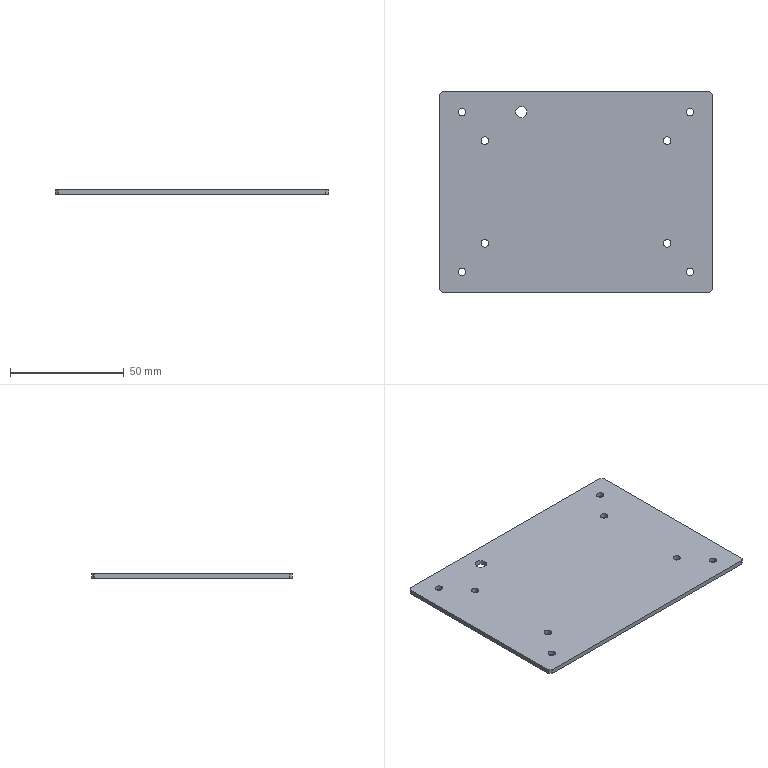Part | SolidWorks | features Extrusion 1, ICE 1 | 1 solid | 28 faces | box 120 x 88 x 2 mm | volume 20938 mm3 | cylinder 22 | plane 6 | commonest cylinder face diameters 3.3 x16 9 x4 5 x2
STEP:
#1=CARTESIAN_POINT('',(-26.5,35.,-1.));
#2=VERTEX_POINT('',#1);
#3=CARTESIAN_POINT('',(-21.5,35.,-1.));
#4=VERTEX_POINT('',#3);
#5=CARTESIAN_POINT('',(-24.,35.,-1.));
#6=DIRECTION('',(0.,0.,1.));
#7=DIRECTION('',(1.,0.,0.));
#8=AXIS2_PLACEMENT_3D('',#5,#6,#7);
#9=CIRCLE('',#8,2.5);
#10=EDGE_CURVE('',#2,#4,#9,.T.);
#11=ORIENTED_EDGE('',*,*,#10,.F.);
#12=CARTESIAN_POINT('',(-26.5,35.,1.));
#13=VERTEX_POINT('',#12);
#14=CARTESIAN_POINT('',(-26.5,35.,-1.));
#15=DIRECTION('',(0.,0.,1.));
#16=VECTOR('',#15,1000.);
#17=LINE('',#14,#16);
#18=EDGE_CURVE('',#2,#13,#17,.T.);
#19=ORIENTED_EDGE('',*,*,#18,.T.);
#20=CARTESIAN_POINT('',(-21.5,35.,1.));
#21=VERTEX_POINT('',#20);
#22=CARTESIAN_POINT('',(-24.,35.,1.));
#23=DIRECTION('',(0.,0.,1.));
#24=DIRECTION('',(1.,0.,0.));
#25=AXIS2_PLACEMENT_3D('',#22,#23,#24);
#26=CIRCLE('',#25,2.5);
#27=EDGE_CURVE('',#13,#21,#26,.T.);
#28=ORIENTED_EDGE('',*,*,#27,.T.);
#29=CARTESIAN_POINT('',(-21.5,35.,-1.));
#30=DIRECTION('',(0.,0.,1.));
#31=VECTOR('',#30,1000.);
#32=LINE('',#29,#31);
#33=EDGE_CURVE('',#4,#21,#32,.T.);
#34=ORIENTED_EDGE('',*,*,#33,.F.);
#35=EDGE_LOOP('',(#11,#19,#28,#34));
#36=FACE_OUTER_BOUND('',#35,.T.);
#37=CARTESIAN_POINT('',(-24.,35.,-1.));
#38=DIRECTION('',(0.,0.,1.));
#39=DIRECTION('',(1.,0.,0.));
#40=AXIS2_PLACEMENT_3D('',#37,#38,#39);
#41=CYLINDRICAL_SURFACE('',#40,2.5);
#42=ADVANCED_FACE('',(#36),#41,.F.);
#43=CARTESIAN_POINT('',(48.35,35.,-1.));
#44=VERTEX_POINT('',#43);
#45=CARTESIAN_POINT('',(51.65,35.,-1.));
#46=VERTEX_POINT('',#45);
#47=CARTESIAN_POINT('',(50.,35.,-1.));
#48=DIRECTION('',(0.,0.,1.));
#49=DIRECTION('',(1.,0.,0.));
#50=AXIS2_PLACEMENT_3D('',#47,#48,#49);
#51=CIRCLE('',#50,1.65);
#52=EDGE_CURVE('',#44,#46,#51,.T.);
#53=ORIENTED_EDGE('',*,*,#52,.F.);
#54=CARTESIAN_POINT('',(48.35,35.,1.));
#55=VERTEX_POINT('',#54);
#56=CARTESIAN_POINT('',(48.35,35.,-1.));
#57=DIRECTION('',(0.,0.,1.));
#58=VECTOR('',#57,1000.);
#59=LINE('',#56,#58);
#60=EDGE_CURVE('',#44,#55,#59,.T.);
#61=ORIENTED_EDGE('',*,*,#60,.T.);
#62=CARTESIAN_POINT('',(51.65,35.,1.));
#63=VERTEX_POINT('',#62);
#64=CARTESIAN_POINT('',(50.,35.,1.));
#65=DIRECTION('',(0.,0.,1.));
#66=DIRECTION('',(1.,0.,0.));
#67=AXIS2_PLACEMENT_3D('',#64,#65,#66);
#68=CIRCLE('',#67,1.65);
#69=EDGE_CURVE('',#55,#63,#68,.T.);
#70=ORIENTED_EDGE('',*,*,#69,.T.);
#71=CARTESIAN_POINT('',(51.65,35.,-1.));
#72=DIRECTION('',(0.,0.,1.));
#73=VECTOR('',#72,1000.);
#74=LINE('',#71,#73);
#75=EDGE_CURVE('',#46,#63,#74,.T.);
#76=ORIENTED_EDGE('',*,*,#75,.F.);
#77=EDGE_LOOP('',(#53,#61,#70,#76));
#78=FACE_OUTER_BOUND('',#77,.T.);
#79=CARTESIAN_POINT('',(50.,35.,-1.));
#80=DIRECTION('',(0.,0.,1.));
#81=DIRECTION('',(1.,0.,0.));
#82=AXIS2_PLACEMENT_3D('',#79,#80,#81);
#83=CYLINDRICAL_SURFACE('',#82,1.65);
#84=ADVANCED_FACE('',(#78),#83,.F.);
#85=CARTESIAN_POINT('',(48.35,-35.,-1.));
#86=VERTEX_POINT('',#85);
#87=CARTESIAN_POINT('',(51.65,-35.,-1.));
#88=VERTEX_POINT('',#87);
#89=CARTESIAN_POINT('',(50.,-35.,-1.));
#90=DIRECTION('',(0.,0.,1.));
#91=DIRECTION('',(1.,0.,0.));
#92=AXIS2_PLACEMENT_3D('',#89,#90,#91);
#93=CIRCLE('',#92,1.65);
#94=EDGE_CURVE('',#86,#88,#93,.T.);
#95=ORIENTED_EDGE('',*,*,#94,.F.);
#96=CARTESIAN_POINT('',(48.35,-35.,1.));
#97=VERTEX_POINT('',#96);
#98=CARTESIAN_POINT('',(48.35,-35.,-1.));
#99=DIRECTION('',(0.,0.,1.));
#100=VECTOR('',#99,1000.);
#101=LINE('',#98,#100);
#102=EDGE_CURVE('',#86,#97,#101,.T.);
#103=ORIENTED_EDGE('',*,*,#102,.T.);
#104=CARTESIAN_POINT('',(51.65,-35.,1.));
#105=VERTEX_POINT('',#104);
#106=CARTESIAN_POINT('',(50.,-35.,1.));
#107=DIRECTION('',(0.,0.,1.));
#108=DIRECTION('',(1.,0.,0.));
#109=AXIS2_PLACEMENT_3D('',#106,#107,#108);
#110=CIRCLE('',#109,1.65);
#111=EDGE_CURVE('',#97,#105,#110,.T.);
#112=ORIENTED_EDGE('',*,*,#111,.T.);
#113=CARTESIAN_POINT('',(51.65,-35.,-1.));
#114=DIRECTION('',(0.,0.,1.));
#115=VECTOR('',#114,1000.);
#116=LINE('',#113,#115);
#117=EDGE_CURVE('',#88,#105,#116,.T.);
#118=ORIENTED_EDGE('',*,*,#117,.F.);
#119=EDGE_LOOP('',(#95,#103,#112,#118));
#120=FACE_OUTER_BOUND('',#119,.T.);
#121=CARTESIAN_POINT('',(50.,-35.,-1.));
#122=DIRECTION('',(0.,0.,1.));
#123=DIRECTION('',(1.,0.,0.));
#124=AXIS2_PLACEMENT_3D('',#121,#122,#123);
#125=CYLINDRICAL_SURFACE('',#124,1.65);
#126=ADVANCED_FACE('',(#120),#125,.F.);
#127=CARTESIAN_POINT('',(-51.65,35.,-1.));
#128=VERTEX_POINT('',#127);
#129=CARTESIAN_POINT('',(-48.35,35.,-1.));
#130=VERTEX_POINT('',#129);
#131=CARTESIAN_POINT('',(-50.,35.,-1.));
#132=DIRECTION('',(0.,0.,1.));
#133=DIRECTION('',(1.,0.,0.));
#134=AXIS2_PLACEMENT_3D('',#131,#132,#133);
#135=CIRCLE('',#134,1.65);
#136=EDGE_CURVE('',#128,#130,#135,.T.);
#137=ORIENTED_EDGE('',*,*,#136,.F.);
#138=CARTESIAN_POINT('',(-51.65,35.,1.));
#139=VERTEX_POINT('',#138);
#140=CARTESIAN_POINT('',(-51.65,35.,-1.));
#141=DIRECTION('',(0.,0.,1.));
#142=VECTOR('',#141,1000.);
#143=LINE('',#140,#142);
#144=EDGE_CURVE('',#128,#139,#143,.T.);
#145=ORIENTED_EDGE('',*,*,#144,.T.);
#146=CARTESIAN_POINT('',(-48.35,35.,1.));
#147=VERTEX_POINT('',#146);
#148=CARTESIAN_POINT('',(-50.,35.,1.));
#149=DIRECTION('',(0.,0.,1.));
#150=DIRECTION('',(1.,0.,0.));
#151=AXIS2_PLACEMENT_3D('',#148,#149,#150);
#152=CIRCLE('',#151,1.65);
#153=EDGE_CURVE('',#139,#147,#152,.T.);
#154=ORIENTED_EDGE('',*,*,#153,.T.);
#155=CARTESIAN_POINT('',(-48.35,35.,-1.));
#156=DIRECTION('',(0.,0.,1.));
#157=VECTOR('',#156,1000.);
#158=LINE('',#155,#157);
#159=EDGE_CURVE('',#130,#147,#158,.T.);
#160=ORIENTED_EDGE('',*,*,#159,.F.);
#161=EDGE_LOOP('',(#137,#145,#154,#160));
#162=FACE_OUTER_BOUND('',#161,.T.);
#163=CARTESIAN_POINT('',(-50.,35.,-1.));
#164=DIRECTION('',(0.,0.,1.));
#165=DIRECTION('',(1.,0.,0.));
#166=AXIS2_PLACEMENT_3D('',#163,#164,#165);
#167=CYLINDRICAL_SURFACE('',#166,1.65);
#168=ADVANCED_FACE('',(#162),#167,.F.);
#169=CARTESIAN_POINT('',(-51.65,-35.,-1.));
#170=VERTEX_POINT('',#169);
#171=CARTESIAN_POINT('',(-48.35,-35.,-1.));
#172=VERTEX_POINT('',#171);
#173=CARTESIAN_POINT('',(-50.,-35.,-1.));
#174=DIRECTION('',(0.,0.,1.));
#175=DIRECTION('',(1.,0.,0.));
#176=AXIS2_PLACEMENT_3D('',#173,#174,#175);
#177=CIRCLE('',#176,1.65);
#178=EDGE_CURVE('',#170,#172,#177,.T.);
#179=ORIENTED_EDGE('',*,*,#178,.F.);
#180=CARTESIAN_POINT('',(-51.65,-35.,1.));
#181=VERTEX_POINT('',#180);
#182=CARTESIAN_POINT('',(-51.65,-35.,-1.));
#183=DIRECTION('',(0.,0.,1.));
#184=VECTOR('',#183,1000.);
#185=LINE('',#182,#184);
#186=EDGE_CURVE('',#170,#181,#185,.T.);
#187=ORIENTED_EDGE('',*,*,#186,.T.);
#188=CARTESIAN_POINT('',(-48.35,-35.,1.));
#189=VERTEX_POINT('',#188);
#190=CARTESIAN_POINT('',(-50.,-35.,1.));
#191=DIRECTION('',(0.,0.,1.));
#192=DIRECTION('',(1.,0.,0.));
#193=AXIS2_PLACEMENT_3D('',#190,#191,#192);
#194=CIRCLE('',#193,1.65);
#195=EDGE_CURVE('',#181,#189,#194,.T.);
#196=ORIENTED_EDGE('',*,*,#195,.T.);
#197=CARTESIAN_POINT('',(-48.35,-35.,-1.));
#198=DIRECTION('',(0.,0.,1.));
#199=VECTOR('',#198,1000.);
#200=LINE('',#197,#199);
#201=EDGE_CURVE('',#172,#189,#200,.T.);
#202=ORIENTED_EDGE('',*,*,#201,.F.);
#203=EDGE_LOOP('',(#179,#187,#196,#202));
#204=FACE_OUTER_BOUND('',#203,.T.);
#205=CARTESIAN_POINT('',(-50.,-35.,-1.));
#206=DIRECTION('',(0.,0.,1.));
#207=DIRECTION('',(1.,0.,0.));
#208=AXIS2_PLACEMENT_3D('',#205,#206,#207);
#209=CYLINDRICAL_SURFACE('',#208,1.65);
#210=ADVANCED_FACE('',(#204),#209,.F.);
#211=CARTESIAN_POINT('',(38.35,22.5,-1.));
#212=VERTEX_POINT('',#211);
#213=CARTESIAN_POINT('',(41.65,22.5,-1.));
#214=VERTEX_POINT('',#213);
#215=CARTESIAN_POINT('',(40.,22.5,-1.));
#216=DIRECTION('',(0.,0.,1.));
#217=DIRECTION('',(1.,0.,0.));
#218=AXIS2_PLACEMENT_3D('',#215,#216,#217);
#219=CIRCLE('',#218,1.65);
#220=EDGE_CURVE('',#212,#214,#219,.T.);
#221=ORIENTED_EDGE('',*,*,#220,.F.);
#222=CARTESIAN_POINT('',(38.35,22.5,1.));
#223=VERTEX_POINT('',#222);
#224=CARTESIAN_POINT('',(38.35,22.5,-1.));
#225=DIRECTION('',(0.,0.,1.));
#226=VECTOR('',#225,1000.);
#227=LINE('',#224,#226);
#228=EDGE_CURVE('',#212,#223,#227,.T.);
#229=ORIENTED_EDGE('',*,*,#228,.T.);
#230=CARTESIAN_POINT('',(41.65,22.5,1.));
#231=VERTEX_POINT('',#230);
#232=CARTESIAN_POINT('',(40.,22.5,1.));
#233=DIRECTION('',(0.,0.,1.));
#234=DIRECTION('',(1.,0.,0.));
#235=AXIS2_PLACEMENT_3D('',#232,#233,#234);
#236=CIRCLE('',#235,1.65);
#237=EDGE_CURVE('',#223,#231,#236,.T.);
#238=ORIENTED_EDGE('',*,*,#237,.T.);
#239=CARTESIAN_POINT('',(41.65,22.5,-1.));
#240=DIRECTION('',(0.,0.,1.));
#241=VECTOR('',#240,1000.);
#242=LINE('',#239,#241);
#243=EDGE_CURVE('',#214,#231,#242,.T.);
#244=ORIENTED_EDGE('',*,*,#243,.F.);
#245=EDGE_LOOP('',(#221,#229,#238,#244));
#246=FACE_OUTER_BOUND('',#245,.T.);
#247=CARTESIAN_POINT('',(40.,22.5,-1.));
#248=DIRECTION('',(0.,0.,1.));
#249=DIRECTION('',(1.,0.,0.));
#250=AXIS2_PLACEMENT_3D('',#247,#248,#249);
#251=CYLINDRICAL_SURFACE('',#250,1.65);
#252=ADVANCED_FACE('',(#246),#251,.F.);
#253=CARTESIAN_POINT('',(38.35,-22.5,-1.));
#254=VERTEX_POINT('',#253);
#255=CARTESIAN_POINT('',(41.65,-22.5,-1.));
#256=VERTEX_POINT('',#255);
#257=CARTESIAN_POINT('',(40.,-22.5,-1.));
#258=DIRECTION('',(0.,0.,1.));
#259=DIRECTION('',(1.,0.,0.));
#260=AXIS2_PLACEMENT_3D('',#257,#258,#259);
#261=CIRCLE('',#260,1.65);
#262=EDGE_CURVE('',#254,#256,#261,.T.);
#263=ORIENTED_EDGE('',*,*,#262,.F.);
#264=CARTESIAN_POINT('',(38.35,-22.5,1.));
#265=VERTEX_POINT('',#264);
#266=CARTESIAN_POINT('',(38.35,-22.5,-1.));
#267=DIRECTION('',(0.,0.,1.));
#268=VECTOR('',#267,1000.);
#269=LINE('',#266,#268);
#270=EDGE_CURVE('',#254,#265,#269,.T.);
#271=ORIENTED_EDGE('',*,*,#270,.T.);
#272=CARTESIAN_POINT('',(41.65,-22.5,1.));
#273=VERTEX_POINT('',#272);
#274=CARTESIAN_POINT('',(40.,-22.5,1.));
#275=DIRECTION('',(0.,0.,1.));
#276=DIRECTION('',(1.,0.,0.));
#277=AXIS2_PLACEMENT_3D('',#274,#275,#276);
#278=CIRCLE('',#277,1.65);
#279=EDGE_CURVE('',#265,#273,#278,.T.);
#280=ORIENTED_EDGE('',*,*,#279,.T.);
#281=CARTESIAN_POINT('',(41.65,-22.5,-1.));
#282=DIRECTION('',(0.,0.,1.));
#283=VECTOR('',#282,1000.);
#284=LINE('',#281,#283);
#285=EDGE_CURVE('',#256,#273,#284,.T.);
#286=ORIENTED_EDGE('',*,*,#285,.F.);
#287=EDGE_LOOP('',(#263,#271,#280,#286));
#288=FACE_OUTER_BOUND('',#287,.T.);
#289=CARTESIAN_POINT('',(40.,-22.5,-1.));
#290=DIRECTION('',(0.,0.,1.));
#291=DIRECTION('',(1.,0.,0.));
#292=AXIS2_PLACEMENT_3D('',#289,#290,#291);
#293=CYLINDRICAL_SURFACE('',#292,1.65);
#294=ADVANCED_FACE('',(#288),#293,.F.);
#295=CARTESIAN_POINT('',(-41.65,22.5,-1.));
#296=VERTEX_POINT('',#295);
#297=CARTESIAN_POINT('',(-38.35,22.5,-1.));
#298=VERTEX_POINT('',#297);
#299=CARTESIAN_POINT('',(-40.,22.5,-1.));
#300=DIRECTION('',(0.,0.,1.));
#301=DIRECTION('',(1.,0.,0.));
#302=AXIS2_PLACEMENT_3D('',#299,#300,#301);
#303=CIRCLE('',#302,1.65);
#304=EDGE_CURVE('',#296,#298,#303,.T.);
#305=ORIENTED_EDGE('',*,*,#304,.F.);
#306=CARTESIAN_POINT('',(-41.65,22.5,1.));
#307=VERTEX_POINT('',#306);
#308=CARTESIAN_POINT('',(-41.65,22.5,-1.));
#309=DIRECTION('',(0.,0.,1.));
#310=VECTOR('',#309,1000.);
#311=LINE('',#308,#310);
#312=EDGE_CURVE('',#296,#307,#311,.T.);
#313=ORIENTED_EDGE('',*,*,#312,.T.);
#314=CARTESIAN_POINT('',(-38.35,22.5,1.));
#315=VERTEX_POINT('',#314);
#316=CARTESIAN_POINT('',(-40.,22.5,1.));
#317=DIRECTION('',(0.,0.,1.));
#318=DIRECTION('',(1.,0.,0.));
#319=AXIS2_PLACEMENT_3D('',#316,#317,#318);
#320=CIRCLE('',#319,1.65);
#321=EDGE_CURVE('',#307,#315,#320,.T.);
#322=ORIENTED_EDGE('',*,*,#321,.T.);
#323=CARTESIAN_POINT('',(-38.35,22.5,-1.));
#324=DIRECTION('',(0.,0.,1.));
#325=VECTOR('',#324,1000.);
#326=LINE('',#323,#325);
#327=EDGE_CURVE('',#298,#315,#326,.T.);
#328=ORIENTED_EDGE('',*,*,#327,.F.);
#329=EDGE_LOOP('',(#305,#313,#322,#328));
#330=FACE_OUTER_BOUND('',#329,.T.);
#331=CARTESIAN_POINT('',(-40.,22.5,-1.));
#332=DIRECTION('',(0.,0.,1.));
#333=DIRECTION('',(1.,0.,0.));
#334=AXIS2_PLACEMENT_3D('',#331,#332,#333);
#335=CYLINDRICAL_SURFACE('',#334,1.65);
#336=ADVANCED_FACE('',(#330),#335,.F.);
#337=CARTESIAN_POINT('',(-41.65,-22.5,-1.));
#338=VERTEX_POINT('',#337);
#339=CARTESIAN_POINT('',(-38.35,-22.5,-1.));
#340=VERTEX_POINT('',#339);
#341=CARTESIAN_POINT('',(-40.,-22.5,-1.));
#342=DIRECTION('',(0.,0.,1.));
#343=DIRECTION('',(1.,0.,0.));
#344=AXIS2_PLACEMENT_3D('',#341,#342,#343);
#345=CIRCLE('',#344,1.65);
#346=EDGE_CURVE('',#338,#340,#345,.T.);
#347=ORIENTED_EDGE('',*,*,#346,.F.);
#348=CARTESIAN_POINT('',(-41.65,-22.5,1.));
#349=VERTEX_POINT('',#348);
#350=CARTESIAN_POINT('',(-41.65,-22.5,-1.));
#351=DIRECTION('',(0.,0.,1.));
#352=VECTOR('',#351,1000.);
#353=LINE('',#350,#352);
#354=EDGE_CURVE('',#338,#349,#353,.T.);
#355=ORIENTED_EDGE('',*,*,#354,.T.);
#356=CARTESIAN_POINT('',(-38.35,-22.5,1.));
#357=VERTEX_POINT('',#356);
#358=CARTESIAN_POINT('',(-40.,-22.5,1.));
#359=DIRECTION('',(0.,0.,1.));
#360=DIRECTION('',(1.,0.,0.));
#361=AXIS2_PLACEMENT_3D('',#358,#359,#360);
#362=CIRCLE('',#361,1.65);
#363=EDGE_CURVE('',#349,#357,#362,.T.);
#364=ORIENTED_EDGE('',*,*,#363,.T.);
#365=CARTESIAN_POINT('',(-38.35,-22.5,-1.));
#366=DIRECTION('',(0.,0.,1.));
#367=VECTOR('',#366,1000.);
#368=LINE('',#365,#367);
#369=EDGE_CURVE('',#340,#357,#368,.T.);
#370=ORIENTED_EDGE('',*,*,#369,.F.);
#371=EDGE_LOOP('',(#347,#355,#364,#370));
#372=FACE_OUTER_BOUND('',#371,.T.);
#373=CARTESIAN_POINT('',(-40.,-22.5,-1.));
#374=DIRECTION('',(0.,0.,1.));
#375=DIRECTION('',(1.,0.,0.));
#376=AXIS2_PLACEMENT_3D('',#373,#374,#375);
#377=CYLINDRICAL_SURFACE('',#376,1.65);
#378=ADVANCED_FACE('',(#372),#377,.F.);
#379=CARTESIAN_POINT('',(-60.,42.969,-1.));
#380=VERTEX_POINT('',#379);
#381=CARTESIAN_POINT('',(-60.,42.969,1.));
#382=VERTEX_POINT('',#381);
#383=CARTESIAN_POINT('',(-60.,42.969,-2.5));
#384=DIRECTION('',(0.,0.,1.));
#385=VECTOR('',#384,1000.);
#386=LINE('',#383,#385);
#387=EDGE_CURVE('',#380,#382,#386,.T.);
#388=ORIENTED_EDGE('',*,*,#387,.F.);
#389=CARTESIAN_POINT('',(-60.,-42.969,-1.));
#390=VERTEX_POINT('',#389);
#391=CARTESIAN_POINT('',(-60.,44.,-1.));
#392=DIRECTION('',(0.,-1.,0.));
#393=VECTOR('',#392,1000.);
#394=LINE('',#391,#393);
#395=EDGE_CURVE('',#380,#390,#394,.T.);
#396=ORIENTED_EDGE('',*,*,#395,.T.);
#397=CARTESIAN_POINT('',(-60.,-42.969,1.));
#398=VERTEX_POINT('',#397);
#399=CARTESIAN_POINT('',(-60.,-42.969,-2.5));
#400=DIRECTION('',(0.,0.,-1.));
#401=VECTOR('',#400,1000.);
#402=LINE('',#399,#401);
#403=EDGE_CURVE('',#398,#390,#402,.T.);
#404=ORIENTED_EDGE('',*,*,#403,.F.);
#405=CARTESIAN_POINT('',(-60.,44.,1.));
#406=DIRECTION('',(0.,-1.,0.));
#407=VECTOR('',#406,1000.);
#408=LINE('',#405,#407);
#409=EDGE_CURVE('',#382,#398,#408,.T.);
#410=ORIENTED_EDGE('',*,*,#409,.F.);
#411=EDGE_LOOP('',(#388,#396,#404,#410));
#412=FACE_OUTER_BOUND('',#411,.T.);
#413=CARTESIAN_POINT('',(-60.,44.,-1.));
#414=DIRECTION('',(-1.,0.,0.));
#415=DIRECTION('',(0.,0.,1.));
#416=AXIS2_PLACEMENT_3D('',#413,#414,#415);
#417=PLANE('',#416);
#418=ADVANCED_FACE('',(#412),#417,.T.);
#419=CARTESIAN_POINT('',(-58.646,44.,1.));
#420=VERTEX_POINT('',#419);
#421=CARTESIAN_POINT('',(-58.646,44.,-1.));
#422=VERTEX_POINT('',#421);
#423=CARTESIAN_POINT('',(-58.646,44.,-2.5));
#424=DIRECTION('',(0.,0.,-1.));
#425=VECTOR('',#424,1000.);
#426=LINE('',#423,#425);
#427=EDGE_CURVE('',#420,#422,#426,.T.);
#428=ORIENTED_EDGE('',*,*,#427,.F.);
#429=CARTESIAN_POINT('',(58.646,44.,1.));
#430=VERTEX_POINT('',#429);
#431=CARTESIAN_POINT('',(60.,44.,1.));
#432=DIRECTION('',(-1.,0.,0.));
#433=VECTOR('',#432,1000.);
#434=LINE('',#431,#433);
#435=EDGE_CURVE('',#430,#420,#434,.T.);
#436=ORIENTED_EDGE('',*,*,#435,.F.);
#437=CARTESIAN_POINT('',(58.646,44.,-1.));
#438=VERTEX_POINT('',#437);
#439=CARTESIAN_POINT('',(58.646,44.,-2.5));
#440=DIRECTION('',(0.,0.,1.));
#441=VECTOR('',#440,1000.);
#442=LINE('',#439,#441);
#443=EDGE_CURVE('',#438,#430,#442,.T.);
#444=ORIENTED_EDGE('',*,*,#443,.F.);
#445=CARTESIAN_POINT('',(60.,44.,-1.));
#446=DIRECTION('',(-1.,0.,0.));
#447=VECTOR('',#446,1000.);
#448=LINE('',#445,#447);
#449=EDGE_CURVE('',#438,#422,#448,.T.);
#450=ORIENTED_EDGE('',*,*,#449,.T.);
#451=EDGE_LOOP('',(#428,#436,#444,#450));
#452=FACE_OUTER_BOUND('',#451,.T.);
#453=CARTESIAN_POINT('',(60.,44.,-1.));
#454=DIRECTION('',(0.,1.,0.));
#455=DIRECTION('',(0.,0.,1.));
#456=AXIS2_PLACEMENT_3D('',#453,#454,#455);
#457=PLANE('',#456);
#458=ADVANCED_FACE('',(#452),#457,.T.);
#459=CARTESIAN_POINT('',(60.,-42.969,-1.));
#460=VERTEX_POINT('',#459);
#461=CARTESIAN_POINT('',(60.,-42.969,1.));
#462=VERTEX_POINT('',#461);
#463=CARTESIAN_POINT('',(60.,-42.969,-2.5));
#464=DIRECTION('',(0.,0.,1.));
#465=VECTOR('',#464,1000.);
#466=LINE('',#463,#465);
#467=EDGE_CURVE('',#460,#462,#466,.T.);
#468=ORIENTED_EDGE('',*,*,#467,.F.);
#469=CARTESIAN_POINT('',(60.,42.969,-1.));
#470=VERTEX_POINT('',#469);
#471=CARTESIAN_POINT('',(60.,-44.,-1.));
#472=DIRECTION('',(0.,1.,0.));
#473=VECTOR('',#472,1000.);
#474=LINE('',#471,#473);
#475=EDGE_CURVE('',#460,#470,#474,.T.);
#476=ORIENTED_EDGE('',*,*,#475,.T.);
#477=CARTESIAN_POINT('',(60.,42.969,1.));
#478=VERTEX_POINT('',#477);
#479=CARTESIAN_POINT('',(60.,42.969,-2.5));
#480=DIRECTION('',(0.,0.,-1.));
#481=VECTOR('',#480,1000.);
#482=LINE('',#479,#481);
#483=EDGE_CURVE('',#478,#470,#482,.T.);
#484=ORIENTED_EDGE('',*,*,#483,.F.);
#485=CARTESIAN_POINT('',(60.,-44.,1.));
#486=DIRECTION('',(0.,1.,0.));
#487=VECTOR('',#486,1000.);
#488=LINE('',#485,#487);
#489=EDGE_CURVE('',#462,#478,#488,.T.);
#490=ORIENTED_EDGE('',*,*,#489,.F.);
#491=EDGE_LOOP('',(#468,#476,#484,#490));
#492=FACE_OUTER_BOUND('',#491,.T.);
#493=CARTESIAN_POINT('',(60.,-44.,-1.));
#494=DIRECTION('',(1.,0.,0.));
#495=DIRECTION('',(0.,0.,-1.));
#496=AXIS2_PLACEMENT_3D('',#493,#494,#495);
#497=PLANE('',#496);
#498=ADVANCED_FACE('',(#492),#497,.T.);
#499=CARTESIAN_POINT('',(58.646,-44.,1.));
#500=VERTEX_POINT('',#499);
#501=CARTESIAN_POINT('',(58.646,-44.,-1.));
#502=VERTEX_POINT('',#501);
#503=CARTESIAN_POINT('',(58.646,-44.,-2.5));
#504=DIRECTION('',(0.,0.,-1.));
#505=VECTOR('',#504,1000.);
#506=LINE('',#503,#505);
#507=EDGE_CURVE('',#500,#502,#506,.T.);
#508=ORIENTED_EDGE('',*,*,#507,.F.);
#509=CARTESIAN_POINT('',(-58.646,-44.,1.));
#510=VERTEX_POINT('',#509);
#511=CARTESIAN_POINT('',(-60.,-44.,1.));
#512=DIRECTION('',(1.,0.,0.));
#513=VECTOR('',#512,1000.);
#514=LINE('',#511,#513);
#515=EDGE_CURVE('',#510,#500,#514,.T.);
#516=ORIENTED_EDGE('',*,*,#515,.F.);
#517=CARTESIAN_POINT('',(-58.646,-44.,-1.));
#518=VERTEX_POINT('',#517);
#519=CARTESIAN_POINT('',(-58.646,-44.,-2.5));
#520=DIRECTION('',(0.,0.,1.));
#521=VECTOR('',#520,1000.);
#522=LINE('',#519,#521);
#523=EDGE_CURVE('',#518,#510,#522,.T.);
#524=ORIENTED_EDGE('',*,*,#523,.F.);
#525=CARTESIAN_POINT('',(-60.,-44.,-1.));
#526=DIRECTION('',(1.,0.,0.));
#527=VECTOR('',#526,1000.);
#528=LINE('',#525,#527);
#529=EDGE_CURVE('',#518,#502,#528,.T.);
#530=ORIENTED_EDGE('',*,*,#529,.T.);
#531=EDGE_LOOP('',(#508,#516,#524,#530));
#532=FACE_OUTER_BOUND('',#531,.T.);
#533=CARTESIAN_POINT('',(-60.,-44.,-1.));
#534=DIRECTION('',(0.,-1.,0.));
#535=DIRECTION('',(0.,0.,-1.));
#536=AXIS2_PLACEMENT_3D('',#533,#534,#535);
#537=PLANE('',#536);
#538=ADVANCED_FACE('',(#532),#537,.T.);
#539=CARTESIAN_POINT('',(-24.,35.,-1.));
#540=DIRECTION('',(0.,0.,1.));
#541=DIRECTION('',(1.,0.,0.));
#542=AXIS2_PLACEMENT_3D('',#539,#540,#541);
#543=CIRCLE('',#542,2.5);
#544=EDGE_CURVE('',#4,#2,#543,.T.);
#545=ORIENTED_EDGE('',*,*,#544,.T.);
#546=ORIENTED_EDGE('',*,*,#10,.T.);
#547=EDGE_LOOP('',(#545,#546));
#548=FACE_BOUND('',#547,.T.);
#549=CARTESIAN_POINT('',(50.,35.,-1.));
#550=DIRECTION('',(0.,0.,1.));
#551=DIRECTION('',(1.,0.,0.));
#552=AXIS2_PLACEMENT_3D('',#549,#550,#551);
#553=CIRCLE('',#552,1.65);
#554=EDGE_CURVE('',#46,#44,#553,.T.);
#555=ORIENTED_EDGE('',*,*,#554,.T.);
#556=ORIENTED_EDGE('',*,*,#52,.T.);
#557=EDGE_LOOP('',(#555,#556));
#558=FACE_BOUND('',#557,.T.);
#559=CARTESIAN_POINT('',(50.,-35.,-1.));
#560=DIRECTION('',(0.,0.,1.));
#561=DIRECTION('',(1.,0.,0.));
#562=AXIS2_PLACEMENT_3D('',#559,#560,#561);
#563=CIRCLE('',#562,1.65);
#564=EDGE_CURVE('',#88,#86,#563,.T.);
#565=ORIENTED_EDGE('',*,*,#564,.T.);
#566=ORIENTED_EDGE('',*,*,#94,.T.);
#567=EDGE_LOOP('',(#565,#566));
#568=FACE_BOUND('',#567,.T.);
#569=CARTESIAN_POINT('',(-50.,35.,-1.));
#570=DIRECTION('',(0.,0.,1.));
#571=DIRECTION('',(1.,0.,0.));
#572=AXIS2_PLACEMENT_3D('',#569,#570,#571);
#573=CIRCLE('',#572,1.65);
#574=EDGE_CURVE('',#130,#128,#573,.T.);
#575=ORIENTED_EDGE('',*,*,#574,.T.);
#576=ORIENTED_EDGE('',*,*,#136,.T.);
#577=EDGE_LOOP('',(#575,#576));
#578=FACE_BOUND('',#577,.T.);
#579=CARTESIAN_POINT('',(-50.,-35.,-1.));
#580=DIRECTION('',(0.,0.,1.));
#581=DIRECTION('',(1.,0.,0.));
#582=AXIS2_PLACEMENT_3D('',#579,#580,#581);
#583=CIRCLE('',#582,1.65);
#584=EDGE_CURVE('',#172,#170,#583,.T.);
#585=ORIENTED_EDGE('',*,*,#584,.T.);
#586=ORIENTED_EDGE('',*,*,#178,.T.);
#587=EDGE_LOOP('',(#585,#586));
#588=FACE_BOUND('',#587,.T.);
#589=CARTESIAN_POINT('',(40.,22.5,-1.));
#590=DIRECTION('',(0.,0.,1.));
#591=DIRECTION('',(1.,0.,0.));
#592=AXIS2_PLACEMENT_3D('',#589,#590,#591);
#593=CIRCLE('',#592,1.65);
#594=EDGE_CURVE('',#214,#212,#593,.T.);
#595=ORIENTED_EDGE('',*,*,#594,.T.);
#596=ORIENTED_EDGE('',*,*,#220,.T.);
#597=EDGE_LOOP('',(#595,#596));
#598=FACE_BOUND('',#597,.T.);
#599=CARTESIAN_POINT('',(40.,-22.5,-1.));
#600=DIRECTION('',(0.,0.,1.));
#601=DIRECTION('',(1.,0.,0.));
#602=AXIS2_PLACEMENT_3D('',#599,#600,#601);
#603=CIRCLE('',#602,1.65);
#604=EDGE_CURVE('',#256,#254,#603,.T.);
#605=ORIENTED_EDGE('',*,*,#604,.T.);
#606=ORIENTED_EDGE('',*,*,#262,.T.);
#607=EDGE_LOOP('',(#605,#606));
#608=FACE_BOUND('',#607,.T.);
#609=CARTESIAN_POINT('',(-40.,22.5,-1.));
#610=DIRECTION('',(0.,0.,1.));
#611=DIRECTION('',(1.,0.,0.));
#612=AXIS2_PLACEMENT_3D('',#609,#610,#611);
#613=CIRCLE('',#612,1.65);
#614=EDGE_CURVE('',#298,#296,#613,.T.);
#615=ORIENTED_EDGE('',*,*,#614,.T.);
#616=ORIENTED_EDGE('',*,*,#304,.T.);
#617=EDGE_LOOP('',(#615,#616));
#618=FACE_BOUND('',#617,.T.);
#619=CARTESIAN_POINT('',(-40.,-22.5,-1.));
#620=DIRECTION('',(0.,0.,1.));
#621=DIRECTION('',(1.,0.,0.));
#622=AXIS2_PLACEMENT_3D('',#619,#620,#621);
#623=CIRCLE('',#622,1.65);
#624=EDGE_CURVE('',#340,#338,#623,.T.);
#625=ORIENTED_EDGE('',*,*,#624,.T.);
#626=ORIENTED_EDGE('',*,*,#346,.T.);
#627=EDGE_LOOP('',(#625,#626));
#628=FACE_BOUND('',#627,.T.);
#629=ORIENTED_EDGE('',*,*,#395,.F.);
#630=CARTESIAN_POINT('',(-62.,47.,-1.));
#631=DIRECTION('',(0.,0.,1.));
#632=DIRECTION('',(1.,0.,0.));
#633=AXIS2_PLACEMENT_3D('',#630,#631,#632);
#634=CIRCLE('',#633,4.5);
#635=EDGE_CURVE('',#380,#422,#634,.T.);
#636=ORIENTED_EDGE('',*,*,#635,.T.);
#637=ORIENTED_EDGE('',*,*,#449,.F.);
#638=CARTESIAN_POINT('',(62.,47.,-1.));
#639=DIRECTION('',(0.,0.,1.));
#640=DIRECTION('',(1.,0.,0.));
#641=AXIS2_PLACEMENT_3D('',#638,#639,#640);
#642=CIRCLE('',#641,4.5);
#643=EDGE_CURVE('',#438,#470,#642,.T.);
#644=ORIENTED_EDGE('',*,*,#643,.T.);
#645=ORIENTED_EDGE('',*,*,#475,.F.);
#646=CARTESIAN_POINT('',(62.,-47.,-1.));
#647=DIRECTION('',(0.,0.,1.));
#648=DIRECTION('',(1.,0.,0.));
#649=AXIS2_PLACEMENT_3D('',#646,#647,#648);
#650=CIRCLE('',#649,4.5);
#651=EDGE_CURVE('',#460,#502,#650,.T.);
#652=ORIENTED_EDGE('',*,*,#651,.T.);
#653=ORIENTED_EDGE('',*,*,#529,.F.);
#654=CARTESIAN_POINT('',(-62.,-47.,-1.));
#655=DIRECTION('',(0.,0.,1.));
#656=DIRECTION('',(1.,0.,0.));
#657=AXIS2_PLACEMENT_3D('',#654,#655,#656);
#658=CIRCLE('',#657,4.5);
#659=EDGE_CURVE('',#518,#390,#658,.T.);
#660=ORIENTED_EDGE('',*,*,#659,.T.);
#661=EDGE_LOOP('',(#629,#636,#637,#644,#645,#652,#653,#660));
#662=FACE_OUTER_BOUND('',#661,.T.);
#663=CARTESIAN_POINT('',(0.,0.,-1.));
#664=DIRECTION('',(0.,0.,1.));
#665=DIRECTION('',(1.,0.,0.));
#666=AXIS2_PLACEMENT_3D('',#663,#664,#665);
#667=PLANE('',#666);
#668=ADVANCED_FACE('',(#548,#558,#568,#578,#588,#598,#608,#618,#628,#662),#667,.F.);
#669=CARTESIAN_POINT('',(-62.,47.,1.));
#670=DIRECTION('',(0.,0.,1.));
#671=DIRECTION('',(1.,0.,0.));
#672=AXIS2_PLACEMENT_3D('',#669,#670,#671);
#673=CIRCLE('',#672,4.5);
#674=EDGE_CURVE('',#382,#420,#673,.T.);
#675=ORIENTED_EDGE('',*,*,#674,.F.);
#676=ORIENTED_EDGE('',*,*,#409,.T.);
#677=CARTESIAN_POINT('',(-62.,-47.,1.));
#678=DIRECTION('',(0.,0.,1.));
#679=DIRECTION('',(1.,0.,0.));
#680=AXIS2_PLACEMENT_3D('',#677,#678,#679);
#681=CIRCLE('',#680,4.5);
#682=EDGE_CURVE('',#510,#398,#681,.T.);
#683=ORIENTED_EDGE('',*,*,#682,.F.);
#684=ORIENTED_EDGE('',*,*,#515,.T.);
#685=CARTESIAN_POINT('',(62.,-47.,1.));
#686=DIRECTION('',(0.,0.,1.));
#687=DIRECTION('',(1.,0.,0.));
#688=AXIS2_PLACEMENT_3D('',#685,#686,#687);
#689=CIRCLE('',#688,4.5);
#690=EDGE_CURVE('',#462,#500,#689,.T.);
#691=ORIENTED_EDGE('',*,*,#690,.F.);
#692=ORIENTED_EDGE('',*,*,#489,.T.);
#693=CARTESIAN_POINT('',(62.,47.,1.));
#694=DIRECTION('',(0.,0.,1.));
#695=DIRECTION('',(1.,0.,0.));
#696=AXIS2_PLACEMENT_3D('',#693,#694,#695);
#697=CIRCLE('',#696,4.5);
#698=EDGE_CURVE('',#430,#478,#697,.T.);
#699=ORIENTED_EDGE('',*,*,#698,.F.);
#700=ORIENTED_EDGE('',*,*,#435,.T.);
#701=EDGE_LOOP('',(#675,#676,#683,#684,#691,#692,#699,#700));
#702=FACE_OUTER_BOUND('',#701,.T.);
#703=CARTESIAN_POINT('',(-24.,35.,1.));
#704=DIRECTION('',(0.,0.,1.));
#705=DIRECTION('',(1.,0.,0.));
#706=AXIS2_PLACEMENT_3D('',#703,#704,#705);
#707=CIRCLE('',#706,2.5);
#708=EDGE_CURVE('',#21,#13,#707,.T.);
#709=ORIENTED_EDGE('',*,*,#708,.F.);
#710=ORIENTED_EDGE('',*,*,#27,.F.);
#711=EDGE_LOOP('',(#709,#710));
#712=FACE_BOUND('',#711,.T.);
#713=CARTESIAN_POINT('',(50.,35.,1.));
#714=DIRECTION('',(0.,0.,1.));
#715=DIRECTION('',(1.,0.,0.));
#716=AXIS2_PLACEMENT_3D('',#713,#714,#715);
#717=CIRCLE('',#716,1.65);
#718=EDGE_CURVE('',#63,#55,#717,.T.);
#719=ORIENTED_EDGE('',*,*,#718,.F.);
#720=ORIENTED_EDGE('',*,*,#69,.F.);
#721=EDGE_LOOP('',(#719,#720));
#722=FACE_BOUND('',#721,.T.);
#723=CARTESIAN_POINT('',(50.,-35.,1.));
#724=DIRECTION('',(0.,0.,1.));
#725=DIRECTION('',(1.,0.,0.));
#726=AXIS2_PLACEMENT_3D('',#723,#724,#725);
#727=CIRCLE('',#726,1.65);
#728=EDGE_CURVE('',#105,#97,#727,.T.);
#729=ORIENTED_EDGE('',*,*,#728,.F.);
#730=ORIENTED_EDGE('',*,*,#111,.F.);
#731=EDGE_LOOP('',(#729,#730));
#732=FACE_BOUND('',#731,.T.);
#733=CARTESIAN_POINT('',(-50.,35.,1.));
#734=DIRECTION('',(0.,0.,1.));
#735=DIRECTION('',(1.,0.,0.));
#736=AXIS2_PLACEMENT_3D('',#733,#734,#735);
#737=CIRCLE('',#736,1.65);
#738=EDGE_CURVE('',#147,#139,#737,.T.);
#739=ORIENTED_EDGE('',*,*,#738,.F.);
#740=ORIENTED_EDGE('',*,*,#153,.F.);
#741=EDGE_LOOP('',(#739,#740));
#742=FACE_BOUND('',#741,.T.);
#743=CARTESIAN_POINT('',(-50.,-35.,1.));
#744=DIRECTION('',(0.,0.,1.));
#745=DIRECTION('',(1.,0.,0.));
#746=AXIS2_PLACEMENT_3D('',#743,#744,#745);
#747=CIRCLE('',#746,1.65);
#748=EDGE_CURVE('',#189,#181,#747,.T.);
#749=ORIENTED_EDGE('',*,*,#748,.F.);
#750=ORIENTED_EDGE('',*,*,#195,.F.);
#751=EDGE_LOOP('',(#749,#750));
#752=FACE_BOUND('',#751,.T.);
#753=CARTESIAN_POINT('',(40.,22.5,1.));
#754=DIRECTION('',(0.,0.,1.));
#755=DIRECTION('',(1.,0.,0.));
#756=AXIS2_PLACEMENT_3D('',#753,#754,#755);
#757=CIRCLE('',#756,1.65);
#758=EDGE_CURVE('',#231,#223,#757,.T.);
#759=ORIENTED_EDGE('',*,*,#758,.F.);
#760=ORIENTED_EDGE('',*,*,#237,.F.);
#761=EDGE_LOOP('',(#759,#760));
#762=FACE_BOUND('',#761,.T.);
#763=CARTESIAN_POINT('',(40.,-22.5,1.));
#764=DIRECTION('',(0.,0.,1.));
#765=DIRECTION('',(1.,0.,0.));
#766=AXIS2_PLACEMENT_3D('',#763,#764,#765);
#767=CIRCLE('',#766,1.65);
#768=EDGE_CURVE('',#273,#265,#767,.T.);
#769=ORIENTED_EDGE('',*,*,#768,.F.);
#770=ORIENTED_EDGE('',*,*,#279,.F.);
#771=EDGE_LOOP('',(#769,#770));
#772=FACE_BOUND('',#771,.T.);
#773=CARTESIAN_POINT('',(-40.,22.5,1.));
#774=DIRECTION('',(0.,0.,1.));
#775=DIRECTION('',(1.,0.,0.));
#776=AXIS2_PLACEMENT_3D('',#773,#774,#775);
#777=CIRCLE('',#776,1.65);
#778=EDGE_CURVE('',#315,#307,#777,.T.);
#779=ORIENTED_EDGE('',*,*,#778,.F.);
#780=ORIENTED_EDGE('',*,*,#321,.F.);
#781=EDGE_LOOP('',(#779,#780));
#782=FACE_BOUND('',#781,.T.);
#783=CARTESIAN_POINT('',(-40.,-22.5,1.));
#784=DIRECTION('',(0.,0.,1.));
#785=DIRECTION('',(1.,0.,0.));
#786=AXIS2_PLACEMENT_3D('',#783,#784,#785);
#787=CIRCLE('',#786,1.65);
#788=EDGE_CURVE('',#357,#349,#787,.T.);
#789=ORIENTED_EDGE('',*,*,#788,.F.);
#790=ORIENTED_EDGE('',*,*,#363,.F.);
#791=EDGE_LOOP('',(#789,#790));
#792=FACE_BOUND('',#791,.T.);
#793=CARTESIAN_POINT('',(0.,0.,1.));
#794=DIRECTION('',(0.,0.,1.));
#795=DIRECTION('',(1.,0.,0.));
#796=AXIS2_PLACEMENT_3D('',#793,#794,#795);
#797=PLANE('',#796);
#798=ADVANCED_FACE('',(#702,#712,#722,#732,#742,#752,#762,#772,#782,#792),#797,.T.);
#799=ORIENTED_EDGE('',*,*,#354,.F.);
#800=ORIENTED_EDGE('',*,*,#624,.F.);
#801=ORIENTED_EDGE('',*,*,#369,.T.);
#802=ORIENTED_EDGE('',*,*,#788,.T.);
#803=EDGE_LOOP('',(#799,#800,#801,#802));
#804=FACE_OUTER_BOUND('',#803,.T.);
#805=CARTESIAN_POINT('',(-40.,-22.5,-1.));
#806=DIRECTION('',(0.,0.,1.));
#807=DIRECTION('',(1.,0.,0.));
#808=AXIS2_PLACEMENT_3D('',#805,#806,#807);
#809=CYLINDRICAL_SURFACE('',#808,1.65);
#810=ADVANCED_FACE('',(#804),#809,.F.);
#811=ORIENTED_EDGE('',*,*,#312,.F.);
#812=ORIENTED_EDGE('',*,*,#614,.F.);
#813=ORIENTED_EDGE('',*,*,#327,.T.);
#814=ORIENTED_EDGE('',*,*,#778,.T.);
#815=EDGE_LOOP('',(#811,#812,#813,#814));
#816=FACE_OUTER_BOUND('',#815,.T.);
#817=CARTESIAN_POINT('',(-40.,22.5,-1.));
#818=DIRECTION('',(0.,0.,1.));
#819=DIRECTION('',(1.,0.,0.));
#820=AXIS2_PLACEMENT_3D('',#817,#818,#819);
#821=CYLINDRICAL_SURFACE('',#820,1.65);
#822=ADVANCED_FACE('',(#816),#821,.F.);
#823=ORIENTED_EDGE('',*,*,#270,.F.);
#824=ORIENTED_EDGE('',*,*,#604,.F.);
#825=ORIENTED_EDGE('',*,*,#285,.T.);
#826=ORIENTED_EDGE('',*,*,#768,.T.);
#827=EDGE_LOOP('',(#823,#824,#825,#826));
#828=FACE_OUTER_BOUND('',#827,.T.);
#829=CARTESIAN_POINT('',(40.,-22.5,-1.));
#830=DIRECTION('',(0.,0.,1.));
#831=DIRECTION('',(1.,0.,0.));
#832=AXIS2_PLACEMENT_3D('',#829,#830,#831);
#833=CYLINDRICAL_SURFACE('',#832,1.65);
#834=ADVANCED_FACE('',(#828),#833,.F.);
#835=ORIENTED_EDGE('',*,*,#228,.F.);
#836=ORIENTED_EDGE('',*,*,#594,.F.);
#837=ORIENTED_EDGE('',*,*,#243,.T.);
#838=ORIENTED_EDGE('',*,*,#758,.T.);
#839=EDGE_LOOP('',(#835,#836,#837,#838));
#840=FACE_OUTER_BOUND('',#839,.T.);
#841=CARTESIAN_POINT('',(40.,22.5,-1.));
#842=DIRECTION('',(0.,0.,1.));
#843=DIRECTION('',(1.,0.,0.));
#844=AXIS2_PLACEMENT_3D('',#841,#842,#843);
#845=CYLINDRICAL_SURFACE('',#844,1.65);
#846=ADVANCED_FACE('',(#840),#845,.F.);
#847=ORIENTED_EDGE('',*,*,#186,.F.);
#848=ORIENTED_EDGE('',*,*,#584,.F.);
#849=ORIENTED_EDGE('',*,*,#201,.T.);
#850=ORIENTED_EDGE('',*,*,#748,.T.);
#851=EDGE_LOOP('',(#847,#848,#849,#850));
#852=FACE_OUTER_BOUND('',#851,.T.);
#853=CARTESIAN_POINT('',(-50.,-35.,-1.));
#854=DIRECTION('',(0.,0.,1.));
#855=DIRECTION('',(1.,0.,0.));
#856=AXIS2_PLACEMENT_3D('',#853,#854,#855);
#857=CYLINDRICAL_SURFACE('',#856,1.65);
#858=ADVANCED_FACE('',(#852),#857,.F.);
#859=ORIENTED_EDGE('',*,*,#144,.F.);
#860=ORIENTED_EDGE('',*,*,#574,.F.);
#861=ORIENTED_EDGE('',*,*,#159,.T.);
#862=ORIENTED_EDGE('',*,*,#738,.T.);
#863=EDGE_LOOP('',(#859,#860,#861,#862));
#864=FACE_OUTER_BOUND('',#863,.T.);
#865=CARTESIAN_POINT('',(-50.,35.,-1.));
#866=DIRECTION('',(0.,0.,1.));
#867=DIRECTION('',(1.,0.,0.));
#868=AXIS2_PLACEMENT_3D('',#865,#866,#867);
#869=CYLINDRICAL_SURFACE('',#868,1.65);
#870=ADVANCED_FACE('',(#864),#869,.F.);
#871=ORIENTED_EDGE('',*,*,#102,.F.);
#872=ORIENTED_EDGE('',*,*,#564,.F.);
#873=ORIENTED_EDGE('',*,*,#117,.T.);
#874=ORIENTED_EDGE('',*,*,#728,.T.);
#875=EDGE_LOOP('',(#871,#872,#873,#874));
#876=FACE_OUTER_BOUND('',#875,.T.);
#877=CARTESIAN_POINT('',(50.,-35.,-1.));
#878=DIRECTION('',(0.,0.,1.));
#879=DIRECTION('',(1.,0.,0.));
#880=AXIS2_PLACEMENT_3D('',#877,#878,#879);
#881=CYLINDRICAL_SURFACE('',#880,1.65);
#882=ADVANCED_FACE('',(#876),#881,.F.);
#883=ORIENTED_EDGE('',*,*,#60,.F.);
#884=ORIENTED_EDGE('',*,*,#554,.F.);
#885=ORIENTED_EDGE('',*,*,#75,.T.);
#886=ORIENTED_EDGE('',*,*,#718,.T.);
#887=EDGE_LOOP('',(#883,#884,#885,#886));
#888=FACE_OUTER_BOUND('',#887,.T.);
#889=CARTESIAN_POINT('',(50.,35.,-1.));
#890=DIRECTION('',(0.,0.,1.));
#891=DIRECTION('',(1.,0.,0.));
#892=AXIS2_PLACEMENT_3D('',#889,#890,#891);
#893=CYLINDRICAL_SURFACE('',#892,1.65);
#894=ADVANCED_FACE('',(#888),#893,.F.);
#895=ORIENTED_EDGE('',*,*,#18,.F.);
#896=ORIENTED_EDGE('',*,*,#544,.F.);
#897=ORIENTED_EDGE('',*,*,#33,.T.);
#898=ORIENTED_EDGE('',*,*,#708,.T.);
#899=EDGE_LOOP('',(#895,#896,#897,#898));
#900=FACE_OUTER_BOUND('',#899,.T.);
#901=CARTESIAN_POINT('',(-24.,35.,-1.));
#902=DIRECTION('',(0.,0.,1.));
#903=DIRECTION('',(1.,0.,0.));
#904=AXIS2_PLACEMENT_3D('',#901,#902,#903);
#905=CYLINDRICAL_SURFACE('',#904,2.5);
#906=ADVANCED_FACE('',(#900),#905,.F.);
#907=ORIENTED_EDGE('',*,*,#523,.T.);
#908=ORIENTED_EDGE('',*,*,#682,.T.);
#909=ORIENTED_EDGE('',*,*,#403,.T.);
#910=ORIENTED_EDGE('',*,*,#659,.F.);
#911=EDGE_LOOP('',(#907,#908,#909,#910));
#912=FACE_OUTER_BOUND('',#911,.T.);
#913=CARTESIAN_POINT('',(-62.,-47.,-2.5));
#914=DIRECTION('',(0.,0.,1.));
#915=DIRECTION('',(1.,0.,0.));
#916=AXIS2_PLACEMENT_3D('',#913,#914,#915);
#917=CYLINDRICAL_SURFACE('',#916,4.5);
#918=ADVANCED_FACE('',(#912),#917,.F.);
#919=ORIENTED_EDGE('',*,*,#443,.T.);
#920=ORIENTED_EDGE('',*,*,#698,.T.);
#921=ORIENTED_EDGE('',*,*,#483,.T.);
#922=ORIENTED_EDGE('',*,*,#643,.F.);
#923=EDGE_LOOP('',(#919,#920,#921,#922));
#924=FACE_OUTER_BOUND('',#923,.T.);
#925=CARTESIAN_POINT('',(62.,47.,-2.5));
#926=DIRECTION('',(0.,0.,1.));
#927=DIRECTION('',(1.,0.,0.));
#928=AXIS2_PLACEMENT_3D('',#925,#926,#927);
#929=CYLINDRICAL_SURFACE('',#928,4.5);
#930=ADVANCED_FACE('',(#924),#929,.F.);
#931=ORIENTED_EDGE('',*,*,#467,.T.);
#932=ORIENTED_EDGE('',*,*,#690,.T.);
#933=ORIENTED_EDGE('',*,*,#507,.T.);
#934=ORIENTED_EDGE('',*,*,#651,.F.);
#935=EDGE_LOOP('',(#931,#932,#933,#934));
#936=FACE_OUTER_BOUND('',#935,.T.);
#937=CARTESIAN_POINT('',(62.,-47.,-2.5));
#938=DIRECTION('',(0.,0.,1.));
#939=DIRECTION('',(1.,0.,0.));
#940=AXIS2_PLACEMENT_3D('',#937,#938,#939);
#941=CYLINDRICAL_SURFACE('',#940,4.5);
#942=ADVANCED_FACE('',(#936),#941,.F.);
#943=ORIENTED_EDGE('',*,*,#387,.T.);
#944=ORIENTED_EDGE('',*,*,#674,.T.);
#945=ORIENTED_EDGE('',*,*,#427,.T.);
#946=ORIENTED_EDGE('',*,*,#635,.F.);
#947=EDGE_LOOP('',(#943,#944,#945,#946));
#948=FACE_OUTER_BOUND('',#947,.T.);
#949=CARTESIAN_POINT('',(-62.,47.,-2.5));
#950=DIRECTION('',(0.,0.,1.));
#951=DIRECTION('',(1.,0.,0.));
#952=AXIS2_PLACEMENT_3D('',#949,#950,#951);
#953=CYLINDRICAL_SURFACE('',#952,4.5);
#954=ADVANCED_FACE('',(#948),#953,.F.);
#955=CLOSED_SHELL('',(#42,#84,#126,#168,#210,#252,#294,#336,#378,#418,#458,#498,#538,#668,#798,#810,#822,#834,#846,#858,#870,#882,#894,#906,#918,#930,#942,#954));
#956=MANIFOLD_SOLID_BREP('',#955);
#957=CARTESIAN_POINT('',(0.,0.,0.));
#958=DIRECTION('',(0.,0.,1.));
#959=DIRECTION('',(1.,0.,0.));
#960=AXIS2_PLACEMENT_3D('',#957,#958,#959);
#961=(LENGTH_UNIT()NAMED_UNIT(*)SI_UNIT(.MILLI.,.METRE.));
#962=UNCERTAINTY_MEASURE_WITH_UNIT(LENGTH_MEASURE(0.00001),#961,'','');
#963=(NAMED_UNIT(*)PLANE_ANGLE_UNIT()SI_UNIT($,.RADIAN.));
#964=(NAMED_UNIT(*)SI_UNIT($,.STERADIAN.)SOLID_ANGLE_UNIT());
#965=(GEOMETRIC_REPRESENTATION_CONTEXT(3)GLOBAL_UNCERTAINTY_ASSIGNED_CONTEXT((#962))GLOBAL_UNIT_ASSIGNED_CONTEXT((#961,#963,#964))REPRESENTATION_CONTEXT('',''));
#966=ADVANCED_BREP_SHAPE_REPRESENTATION('',(#956,#960),#965);